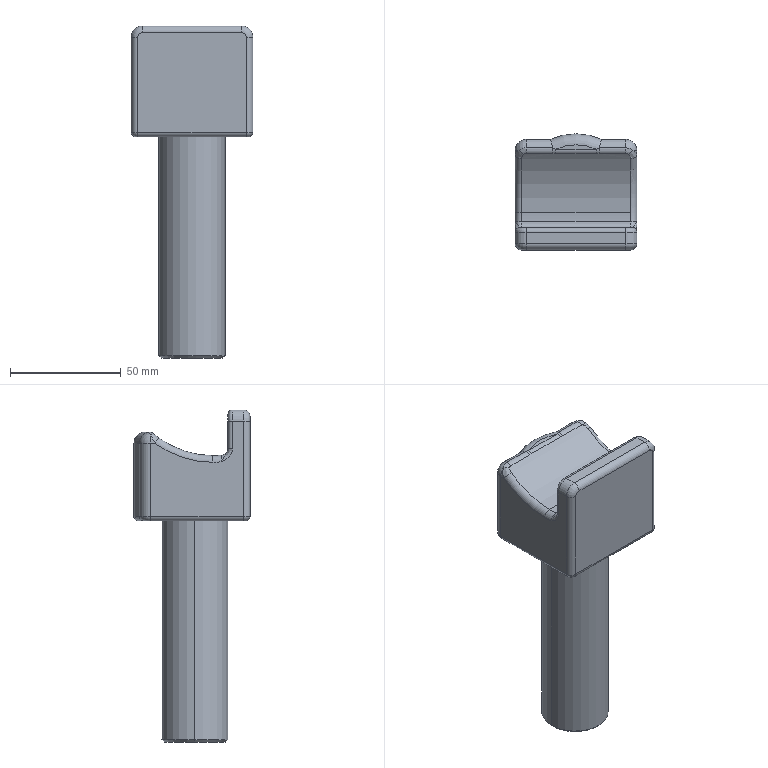Part | SolidWorks | features Fillet 9, ICE 4, Chamfer 1, Extrusion 1 | 1 solid | 65 faces | box 55 x 52.5 x 150 mm | volume 171259 mm3 | cylinder 28 | torus 13 | plane 10 | spline 10 | cone 2 | sphere 2 | commonest cylinder face diameters 4 x8 10 x8 6 x7 30 x2 82.201 x2 55 x1